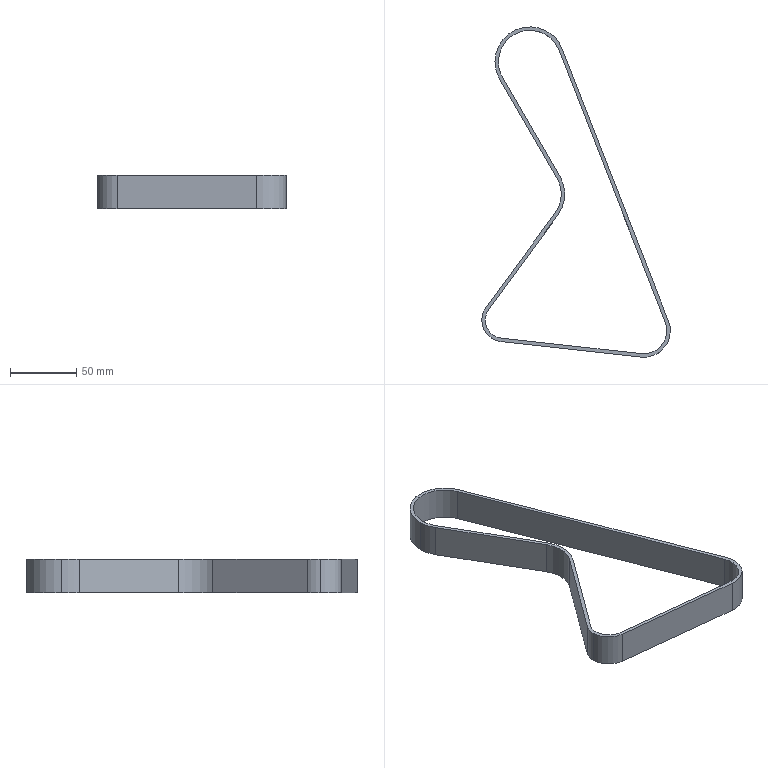Part | STEP file | Belt 5-2^ traction group | 1 solid | 22 faces | box 142.32 x 249.37 x 25 mm | volume 44730 mm3 | cylinder 12 | plane 10 | commonest cylinder face diameters 47.48 x3 52.72 x3 27.38 x2 32.62 x2 34.78 x1 40.02 x1